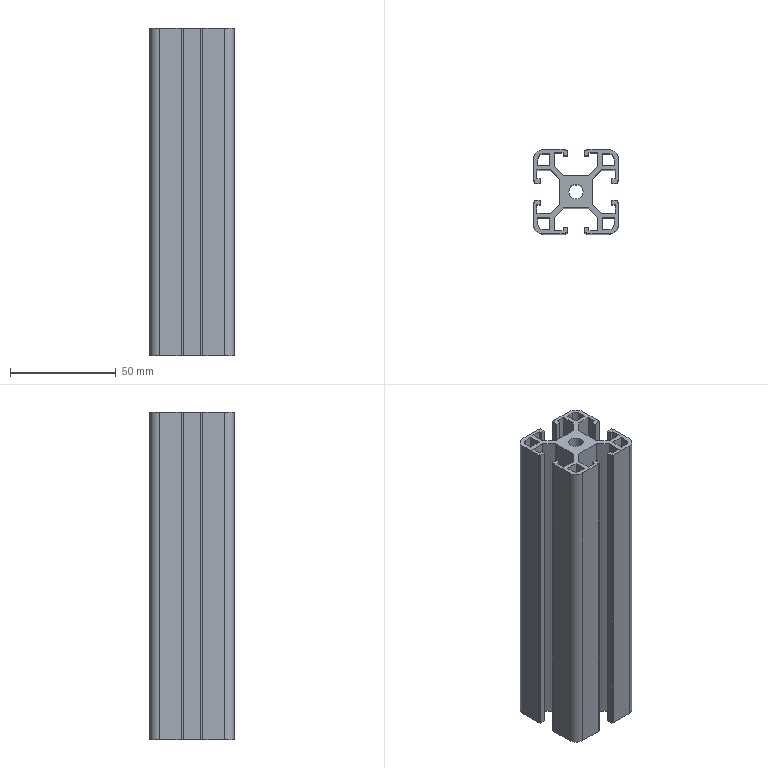Part | NX | features DATUM_CSYS 2, EXTRUDE 1, SKETCH 1 | 1 solid | 103 faces | box 40 x 40 x 155 mm | volume 89365 mm3 | plane 94 | cylinder 9 | commonest cylinder face diameters 5 x4 9 x4 6.8 x1